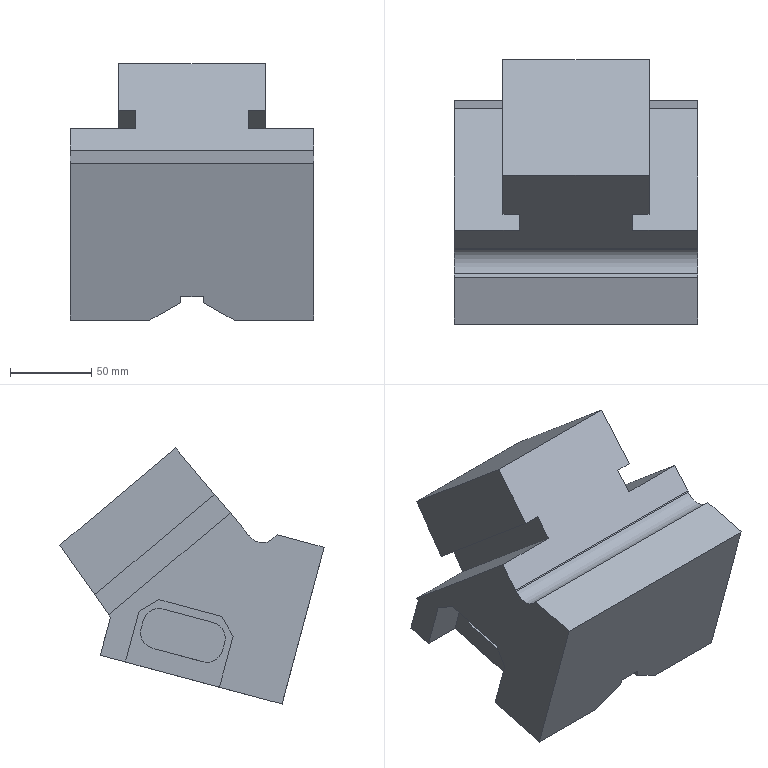Part | NX | features solid 2 | 1 solid | 58 faces | box 150 x 162.858 x 157.827 mm | volume 1676747 mm3 | plane 48 | cylinder 9 | spline 1 | commonest cylinder face diameters 20 x9